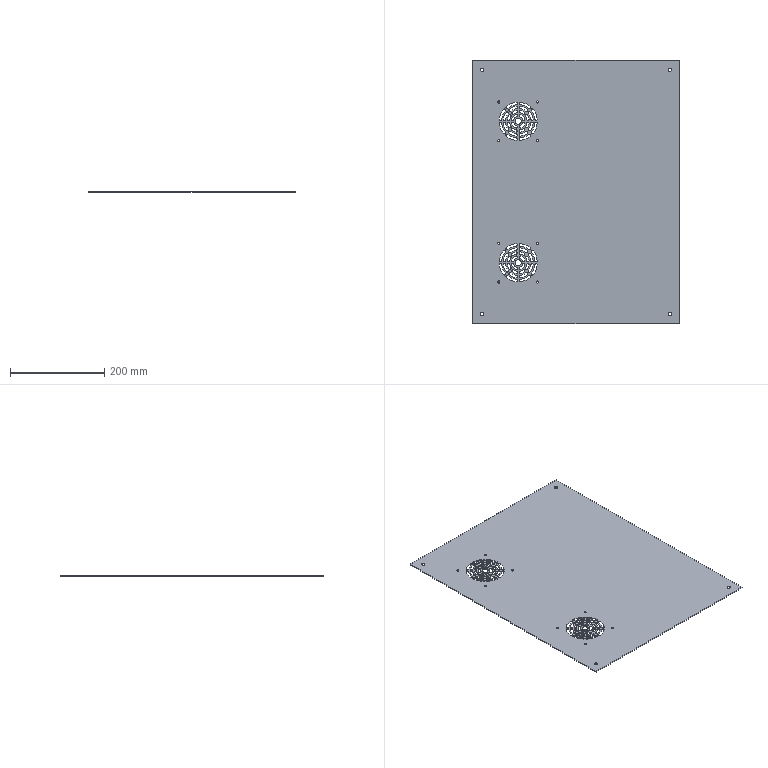Part | STEP file | 09-26 closing plate c (Default) | 1 solid | 314 faces | box 438 x 558 x 1.5 mm | volume 358211 mm3 | cylinder 308 | plane 6 | commonest cylinder face diameters 5 x168 4.5 x16 37 x16 47 x16 54 x16 64 x16